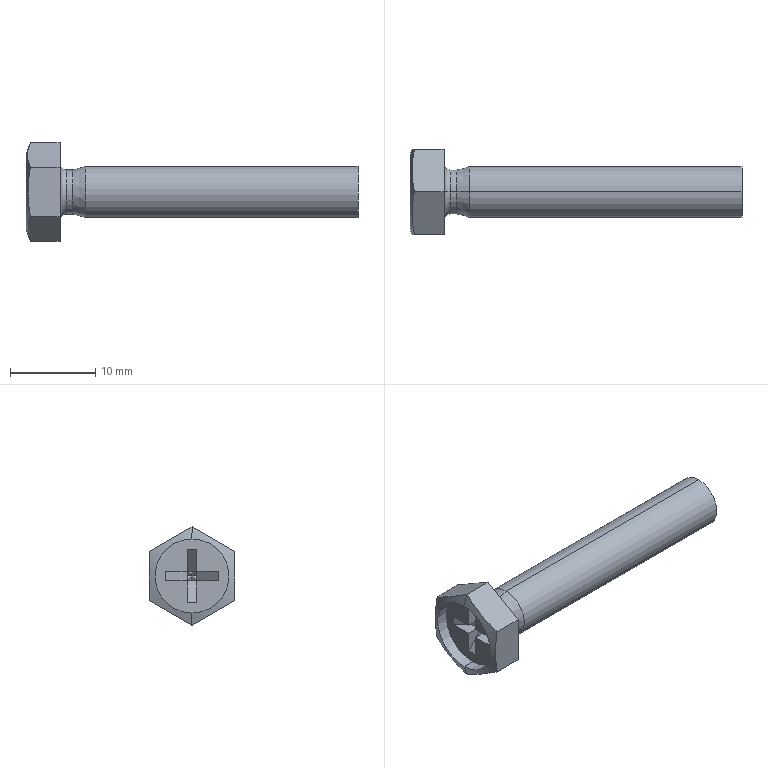Part | SolidWorks | features Cut 2, RevCut 2, CirPattern 1, Extrusion 1, LPattern 1, Revolution 1 | 1 solid | 45 faces | box 39 x 10 x 11.547 mm | volume 1217 mm3 | plane 33 | cylinder 6 | cone 4 | torus 2 | commonest cylinder face diameters 5.2 x2 6 x2 8.7 x2
STEP:
#1=CARTESIAN_POINT('',(1.4,0.,-4.35));
#2=VERTEX_POINT('',#1);
#3=CARTESIAN_POINT('',(1.4,0.,4.35));
#4=VERTEX_POINT('',#3);
#5=CARTESIAN_POINT('',(1.4,0.,0.));
#6=DIRECTION('',(-1.,0.,0.));
#7=DIRECTION('',(0.,0.,1.));
#8=AXIS2_PLACEMENT_3D('',#5,#6,#7);
#9=CIRCLE('',#8,4.35);
#10=EDGE_CURVE('',#2,#4,#9,.T.);
#11=ORIENTED_EDGE('',*,*,#10,.F.);
#12=CARTESIAN_POINT('',(0.,0.,-4.35));
#13=VERTEX_POINT('',#12);
#14=CARTESIAN_POINT('',(1.4,0.,-4.35));
#15=DIRECTION('',(-1.,0.,0.));
#16=VECTOR('',#15,1000.);
#17=LINE('',#14,#16);
#18=EDGE_CURVE('',#2,#13,#17,.T.);
#19=ORIENTED_EDGE('',*,*,#18,.T.);
#20=CARTESIAN_POINT('',(0.,0.,4.35));
#21=VERTEX_POINT('',#20);
#22=CARTESIAN_POINT('',(0.,0.,0.));
#23=DIRECTION('',(-1.,0.,0.));
#24=DIRECTION('',(0.,0.,1.));
#25=AXIS2_PLACEMENT_3D('',#22,#23,#24);
#26=CIRCLE('',#25,4.35);
#27=EDGE_CURVE('',#13,#21,#26,.T.);
#28=ORIENTED_EDGE('',*,*,#27,.T.);
#29=CARTESIAN_POINT('',(1.4,0.,4.35));
#30=DIRECTION('',(-1.,0.,0.));
#31=VECTOR('',#30,1000.);
#32=LINE('',#29,#31);
#33=EDGE_CURVE('',#4,#21,#32,.T.);
#34=ORIENTED_EDGE('',*,*,#33,.F.);
#35=EDGE_LOOP('',(#11,#19,#28,#34));
#36=FACE_OUTER_BOUND('',#35,.T.);
#37=CARTESIAN_POINT('',(1.4,0.,0.));
#38=DIRECTION('',(-1.,0.,0.));
#39=DIRECTION('',(0.,0.,1.));
#40=AXIS2_PLACEMENT_3D('',#37,#38,#39);
#41=CYLINDRICAL_SURFACE('',#40,4.35);
#42=ADVANCED_FACE('',(#36),#41,.F.);
#43=CARTESIAN_POINT('',(0.,0.,0.));
#44=DIRECTION('',(-1.,0.,0.));
#45=DIRECTION('',(0.,0.,1.));
#46=AXIS2_PLACEMENT_3D('',#43,#44,#45);
#47=CIRCLE('',#46,4.35);
#48=EDGE_CURVE('',#21,#13,#47,.T.);
#49=ORIENTED_EDGE('',*,*,#48,.F.);
#50=CARTESIAN_POINT('',(0.5181,0.,5.774));
#51=VERTEX_POINT('',#50);
#52=CARTESIAN_POINT('',(0.,0.,4.35));
#53=DIRECTION('',(0.342,0.,0.9397));
#54=VECTOR('',#53,1000.);
#55=LINE('',#52,#54);
#56=EDGE_CURVE('',#21,#51,#55,.T.);
#57=ORIENTED_EDGE('',*,*,#56,.T.);
#58=CARTESIAN_POINT('',(0.5181,5.,2.887));
#59=VERTEX_POINT('',#58);
#60=CARTESIAN_POINT('',(0.5181,0.,5.774));
#61=CARTESIAN_POINT('',(0.343,0.8333,5.292));
#62=CARTESIAN_POINT('',(0.1302,2.5,4.33));
#63=CARTESIAN_POINT('',(0.343,4.167,3.368));
#64=CARTESIAN_POINT('',(0.5181,5.,2.887));
#65=B_SPLINE_CURVE_WITH_KNOTS('',3,(#60,#61,#62,#63,#64),.UNSPECIFIED.,.F.,.F.,(4,1,4),(0.000000231,0.002887,0.005774),.UNSPECIFIED.);
#66=EDGE_CURVE('',#51,#59,#65,.T.);
#67=ORIENTED_EDGE('',*,*,#66,.T.);
#68=CARTESIAN_POINT('',(0.5181,5.,-2.887));
#69=VERTEX_POINT('',#68);
#70=CARTESIAN_POINT('',(0.5181,5.,2.887));
#71=CARTESIAN_POINT('',(0.3437,5.,1.928));
#72=CARTESIAN_POINT('',(0.2369,5.,0.9672));
#73=CARTESIAN_POINT('',(0.2364,5.,-0.4771));
#74=CARTESIAN_POINT('',(0.2621,5.,-0.9591));
#75=CARTESIAN_POINT('',(0.3594,5.,-1.924));
#76=CARTESIAN_POINT('',(0.431,5.,-2.408));
#77=CARTESIAN_POINT('',(0.5181,5.,-2.887));
#78=B_SPLINE_CURVE_WITH_KNOTS('',3,(#70,#71,#72,#73,#74,#75,#76,#77),.UNSPECIFIED.,.F.,.F.,(4,2,2,4),(0.0105,0.01341,0.01486,0.01631),.UNSPECIFIED.);
#79=EDGE_CURVE('',#59,#69,#78,.T.);
#80=ORIENTED_EDGE('',*,*,#79,.T.);
#81=CARTESIAN_POINT('',(0.5181,0.,-5.774));
#82=VERTEX_POINT('',#81);
#83=CARTESIAN_POINT('',(0.5181,5.,-2.887));
#84=CARTESIAN_POINT('',(0.343,4.167,-3.368));
#85=CARTESIAN_POINT('',(0.1302,2.5,-4.33));
#86=CARTESIAN_POINT('',(0.343,0.8333,-5.292));
#87=CARTESIAN_POINT('',(0.5181,0.,-5.774));
#88=B_SPLINE_CURVE_WITH_KNOTS('',3,(#83,#84,#85,#86,#87),.UNSPECIFIED.,.F.,.F.,(4,1,4),(0.000000231,0.002887,0.005774),.UNSPECIFIED.);
#89=EDGE_CURVE('',#69,#82,#88,.T.);
#90=ORIENTED_EDGE('',*,*,#89,.T.);
#91=CARTESIAN_POINT('',(0.,0.,-4.35));
#92=DIRECTION('',(0.342,0.,-0.9397));
#93=VECTOR('',#92,1000.);
#94=LINE('',#91,#93);
#95=EDGE_CURVE('',#13,#82,#94,.T.);
#96=ORIENTED_EDGE('',*,*,#95,.F.);
#97=EDGE_LOOP('',(#49,#57,#67,#80,#90,#96));
#98=FACE_OUTER_BOUND('',#97,.T.);
#99=CARTESIAN_POINT('',(0.,0.,0.));
#100=DIRECTION('',(1.,0.,0.));
#101=DIRECTION('',(0.,0.,-1.));
#102=AXIS2_PLACEMENT_3D('',#99,#100,#101);
#103=CONICAL_SURFACE('',#102,4.35,1.222);
#104=ADVANCED_FACE('',(#98),#103,.T.);
#105=CARTESIAN_POINT('',(4.,0.,-3.4));
#106=VERTEX_POINT('',#105);
#107=CARTESIAN_POINT('',(4.,0.,3.4));
#108=VERTEX_POINT('',#107);
#109=CARTESIAN_POINT('',(4.,0.,0.));
#110=DIRECTION('',(-1.,0.,0.));
#111=DIRECTION('',(0.,0.,1.));
#112=AXIS2_PLACEMENT_3D('',#109,#110,#111);
#113=CIRCLE('',#112,3.4);
#114=EDGE_CURVE('',#106,#108,#113,.T.);
#115=ORIENTED_EDGE('',*,*,#114,.F.);
#116=CARTESIAN_POINT('',(4.8,0.,-2.6));
#117=VERTEX_POINT('',#116);
#118=CARTESIAN_POINT('',(4.8,0.,-3.4));
#119=DIRECTION('',(0.,1.,0.));
#120=DIRECTION('',(0.,0.,1.));
#121=AXIS2_PLACEMENT_3D('',#118,#119,#120);
#122=CIRCLE('',#121,0.8);
#123=EDGE_CURVE('',#106,#117,#122,.T.);
#124=ORIENTED_EDGE('',*,*,#123,.T.);
#125=CARTESIAN_POINT('',(4.8,0.,2.6));
#126=VERTEX_POINT('',#125);
#127=CARTESIAN_POINT('',(4.8,0.,0.));
#128=DIRECTION('',(-1.,0.,0.));
#129=DIRECTION('',(0.,0.,1.));
#130=AXIS2_PLACEMENT_3D('',#127,#128,#129);
#131=CIRCLE('',#130,2.6);
#132=EDGE_CURVE('',#117,#126,#131,.T.);
#133=ORIENTED_EDGE('',*,*,#132,.T.);
#134=CARTESIAN_POINT('',(4.8,0.,3.4));
#135=DIRECTION('',(0.,-1.,0.));
#136=DIRECTION('',(0.,0.,-1.));
#137=AXIS2_PLACEMENT_3D('',#134,#135,#136);
#138=CIRCLE('',#137,0.8);
#139=EDGE_CURVE('',#108,#126,#138,.T.);
#140=ORIENTED_EDGE('',*,*,#139,.F.);
#141=EDGE_LOOP('',(#115,#124,#133,#140));
#142=FACE_OUTER_BOUND('',#141,.T.);
#143=CARTESIAN_POINT('',(4.8,0.,0.));
#144=DIRECTION('',(-1.,0.,0.));
#145=DIRECTION('',(0.,0.,1.));
#146=AXIS2_PLACEMENT_3D('',#143,#144,#145);
#147=TOROIDAL_SURFACE('',#146,3.4,0.8);
#148=ADVANCED_FACE('',(#142),#147,.F.);
#149=CARTESIAN_POINT('',(5.507,0.,2.6));
#150=VERTEX_POINT('',#149);
#151=CARTESIAN_POINT('',(5.507,0.,-2.6));
#152=VERTEX_POINT('',#151);
#153=CARTESIAN_POINT('',(5.507,0.,0.));
#154=DIRECTION('',(-1.,0.,0.));
#155=DIRECTION('',(0.,0.,1.));
#156=AXIS2_PLACEMENT_3D('',#153,#154,#155);
#157=CIRCLE('',#156,2.6);
#158=EDGE_CURVE('',#150,#152,#157,.T.);
#159=ORIENTED_EDGE('',*,*,#158,.T.);
#160=CARTESIAN_POINT('',(0.,0.,-2.6));
#161=DIRECTION('',(-1.,0.,0.));
#162=VECTOR('',#161,1000.);
#163=LINE('',#160,#162);
#164=EDGE_CURVE('',#152,#117,#163,.T.);
#165=ORIENTED_EDGE('',*,*,#164,.T.);
#166=CARTESIAN_POINT('',(4.8,0.,0.));
#167=DIRECTION('',(-1.,0.,0.));
#168=DIRECTION('',(0.,0.,1.));
#169=AXIS2_PLACEMENT_3D('',#166,#167,#168);
#170=CIRCLE('',#169,2.6);
#171=EDGE_CURVE('',#126,#117,#170,.T.);
#172=ORIENTED_EDGE('',*,*,#171,.F.);
#173=CARTESIAN_POINT('',(0.,0.,2.6));
#174=DIRECTION('',(-1.,0.,0.));
#175=VECTOR('',#174,1000.);
#176=LINE('',#173,#175);
#177=EDGE_CURVE('',#150,#126,#176,.T.);
#178=ORIENTED_EDGE('',*,*,#177,.F.);
#179=EDGE_LOOP('',(#159,#165,#172,#178));
#180=FACE_OUTER_BOUND('',#179,.T.);
#181=CARTESIAN_POINT('',(0.,0.,0.));
#182=DIRECTION('',(-1.,0.,0.));
#183=DIRECTION('',(0.,0.,1.));
#184=AXIS2_PLACEMENT_3D('',#181,#182,#183);
#185=CYLINDRICAL_SURFACE('',#184,2.6);
#186=ADVANCED_FACE('',(#180),#185,.T.);
#187=ORIENTED_EDGE('',*,*,#158,.F.);
#188=CARTESIAN_POINT('',(7.,0.,3.));
#189=VERTEX_POINT('',#188);
#190=CARTESIAN_POINT('',(7.,0.,3.));
#191=DIRECTION('',(0.9659,0.,0.2588));
#192=VECTOR('',#191,1000.);
#193=LINE('',#190,#192);
#194=EDGE_CURVE('',#150,#189,#193,.T.);
#195=ORIENTED_EDGE('',*,*,#194,.T.);
#196=CARTESIAN_POINT('',(7.,0.,-3.));
#197=VERTEX_POINT('',#196);
#198=CARTESIAN_POINT('',(7.,0.,0.));
#199=DIRECTION('',(-1.,0.,0.));
#200=DIRECTION('',(0.,0.,1.));
#201=AXIS2_PLACEMENT_3D('',#198,#199,#200);
#202=CIRCLE('',#201,3.);
#203=EDGE_CURVE('',#189,#197,#202,.T.);
#204=ORIENTED_EDGE('',*,*,#203,.T.);
#205=CARTESIAN_POINT('',(7.,0.,-3.));
#206=DIRECTION('',(0.9659,0.,-0.2588));
#207=VECTOR('',#206,1000.);
#208=LINE('',#205,#207);
#209=EDGE_CURVE('',#152,#197,#208,.T.);
#210=ORIENTED_EDGE('',*,*,#209,.F.);
#211=EDGE_LOOP('',(#187,#195,#204,#210));
#212=FACE_OUTER_BOUND('',#211,.T.);
#213=CARTESIAN_POINT('',(7.,0.,0.));
#214=DIRECTION('',(1.,0.,0.));
#215=DIRECTION('',(0.,0.,-1.));
#216=AXIS2_PLACEMENT_3D('',#213,#214,#215);
#217=CONICAL_SURFACE('',#216,3.,0.2618);
#218=ADVANCED_FACE('',(#212),#217,.T.);
#219=CARTESIAN_POINT('',(39.,0.,3.));
#220=VERTEX_POINT('',#219);
#221=CARTESIAN_POINT('',(39.,0.,-3.));
#222=VERTEX_POINT('',#221);
#223=CARTESIAN_POINT('',(39.,0.,0.));
#224=DIRECTION('',(-1.,0.,0.));
#225=DIRECTION('',(0.,0.,1.));
#226=AXIS2_PLACEMENT_3D('',#223,#224,#225);
#227=CIRCLE('',#226,3.);
#228=EDGE_CURVE('',#220,#222,#227,.T.);
#229=ORIENTED_EDGE('',*,*,#228,.T.);
#230=CARTESIAN_POINT('',(0.,0.,-3.));
#231=DIRECTION('',(-1.,0.,0.));
#232=VECTOR('',#231,1000.);
#233=LINE('',#230,#232);
#234=EDGE_CURVE('',#222,#197,#233,.T.);
#235=ORIENTED_EDGE('',*,*,#234,.T.);
#236=ORIENTED_EDGE('',*,*,#203,.F.);
#237=CARTESIAN_POINT('',(0.,0.,3.));
#238=DIRECTION('',(-1.,0.,0.));
#239=VECTOR('',#238,1000.);
#240=LINE('',#237,#239);
#241=EDGE_CURVE('',#220,#189,#240,.T.);
#242=ORIENTED_EDGE('',*,*,#241,.F.);
#243=EDGE_LOOP('',(#229,#235,#236,#242));
#244=FACE_OUTER_BOUND('',#243,.T.);
#245=CARTESIAN_POINT('',(0.,0.,0.));
#246=DIRECTION('',(-1.,0.,0.));
#247=DIRECTION('',(0.,0.,1.));
#248=AXIS2_PLACEMENT_3D('',#245,#246,#247);
#249=CYLINDRICAL_SURFACE('',#248,3.);
#250=ADVANCED_FACE('',(#244),#249,.T.);
#251=CARTESIAN_POINT('',(1.4,0.,0.));
#252=DIRECTION('',(-1.,0.,0.));
#253=DIRECTION('',(0.,0.,1.));
#254=AXIS2_PLACEMENT_3D('',#251,#252,#253);
#255=CIRCLE('',#254,4.35);
#256=EDGE_CURVE('',#4,#2,#255,.T.);
#257=ORIENTED_EDGE('',*,*,#256,.T.);
#258=ORIENTED_EDGE('',*,*,#10,.T.);
#259=EDGE_LOOP('',(#257,#258));
#260=FACE_OUTER_BOUND('',#259,.T.);
#261=CARTESIAN_POINT('',(1.4,3.1,0.572));
#262=VERTEX_POINT('',#261);
#263=CARTESIAN_POINT('',(1.4,3.1,-0.572));
#264=VERTEX_POINT('',#263);
#265=CARTESIAN_POINT('',(1.4,3.1,0.));
#266=DIRECTION('',(0.,0.,-1.));
#267=VECTOR('',#266,1000.);
#268=LINE('',#265,#267);
#269=EDGE_CURVE('',#262,#264,#268,.T.);
#270=ORIENTED_EDGE('',*,*,#269,.F.);
#271=CARTESIAN_POINT('',(1.4,0.572,0.572));
#272=VERTEX_POINT('',#271);
#273=CARTESIAN_POINT('',(1.4,0.,0.572));
#274=DIRECTION('',(0.,-1.,0.));
#275=VECTOR('',#274,1000.);
#276=LINE('',#273,#275);
#277=EDGE_CURVE('',#262,#272,#276,.T.);
#278=ORIENTED_EDGE('',*,*,#277,.T.);
#279=CARTESIAN_POINT('',(1.4,0.572,3.1));
#280=VERTEX_POINT('',#279);
#281=CARTESIAN_POINT('',(1.4,0.572,0.));
#282=DIRECTION('',(0.,0.,-1.));
#283=VECTOR('',#282,1000.);
#284=LINE('',#281,#283);
#285=EDGE_CURVE('',#280,#272,#284,.T.);
#286=ORIENTED_EDGE('',*,*,#285,.F.);
#287=CARTESIAN_POINT('',(1.4,-0.572,3.1));
#288=VERTEX_POINT('',#287);
#289=CARTESIAN_POINT('',(1.4,0.,3.1));
#290=DIRECTION('',(0.,1.,0.));
#291=VECTOR('',#290,1000.);
#292=LINE('',#289,#291);
#293=EDGE_CURVE('',#288,#280,#292,.T.);
#294=ORIENTED_EDGE('',*,*,#293,.F.);
#295=CARTESIAN_POINT('',(1.4,-0.572,0.572));
#296=VERTEX_POINT('',#295);
#297=CARTESIAN_POINT('',(1.4,-0.572,0.));
#298=DIRECTION('',(0.,0.,-1.));
#299=VECTOR('',#298,1000.);
#300=LINE('',#297,#299);
#301=EDGE_CURVE('',#288,#296,#300,.T.);
#302=ORIENTED_EDGE('',*,*,#301,.T.);
#303=CARTESIAN_POINT('',(1.4,-3.1,0.572));
#304=VERTEX_POINT('',#303);
#305=CARTESIAN_POINT('',(1.4,0.,0.572));
#306=DIRECTION('',(0.,-1.,0.));
#307=VECTOR('',#306,1000.);
#308=LINE('',#305,#307);
#309=EDGE_CURVE('',#296,#304,#308,.T.);
#310=ORIENTED_EDGE('',*,*,#309,.T.);
#311=CARTESIAN_POINT('',(1.4,-3.1,-0.572));
#312=VERTEX_POINT('',#311);
#313=CARTESIAN_POINT('',(1.4,-3.1,0.));
#314=DIRECTION('',(0.,0.,1.));
#315=VECTOR('',#314,1000.);
#316=LINE('',#313,#315);
#317=EDGE_CURVE('',#312,#304,#316,.T.);
#318=ORIENTED_EDGE('',*,*,#317,.F.);
#319=CARTESIAN_POINT('',(1.4,-0.572,-0.572));
#320=VERTEX_POINT('',#319);
#321=CARTESIAN_POINT('',(1.4,0.,-0.572));
#322=DIRECTION('',(0.,-1.,0.));
#323=VECTOR('',#322,1000.);
#324=LINE('',#321,#323);
#325=EDGE_CURVE('',#320,#312,#324,.T.);
#326=ORIENTED_EDGE('',*,*,#325,.F.);
#327=CARTESIAN_POINT('',(1.4,-0.572,-3.1));
#328=VERTEX_POINT('',#327);
#329=CARTESIAN_POINT('',(1.4,-0.572,0.));
#330=DIRECTION('',(0.,0.,-1.));
#331=VECTOR('',#330,1000.);
#332=LINE('',#329,#331);
#333=EDGE_CURVE('',#320,#328,#332,.T.);
#334=ORIENTED_EDGE('',*,*,#333,.T.);
#335=CARTESIAN_POINT('',(1.4,0.572,-3.1));
#336=VERTEX_POINT('',#335);
#337=CARTESIAN_POINT('',(1.4,0.,-3.1));
#338=DIRECTION('',(0.,-1.,0.));
#339=VECTOR('',#338,1000.);
#340=LINE('',#337,#339);
#341=EDGE_CURVE('',#336,#328,#340,.T.);
#342=ORIENTED_EDGE('',*,*,#341,.F.);
#343=CARTESIAN_POINT('',(1.4,0.572,-0.572));
#344=VERTEX_POINT('',#343);
#345=CARTESIAN_POINT('',(1.4,0.572,0.));
#346=DIRECTION('',(0.,0.,-1.));
#347=VECTOR('',#346,1000.);
#348=LINE('',#345,#347);
#349=EDGE_CURVE('',#344,#336,#348,.T.);
#350=ORIENTED_EDGE('',*,*,#349,.F.);
#351=CARTESIAN_POINT('',(1.4,0.,-0.572));
#352=DIRECTION('',(0.,-1.,0.));
#353=VECTOR('',#352,1000.);
#354=LINE('',#351,#353);
#355=EDGE_CURVE('',#264,#344,#354,.T.);
#356=ORIENTED_EDGE('',*,*,#355,.F.);
#357=EDGE_LOOP('',(#270,#278,#286,#294,#302,#310,#318,#326,#334,#342,#350,#356));
#358=FACE_BOUND('',#357,.T.);
#359=CARTESIAN_POINT('',(1.4,0.,0.));
#360=DIRECTION('',(-1.,0.,0.));
#361=DIRECTION('',(0.,0.,1.));
#362=AXIS2_PLACEMENT_3D('',#359,#360,#361);
#363=PLANE('',#362);
#364=ADVANCED_FACE('',(#260,#358),#363,.T.);
#365=CARTESIAN_POINT('',(3.732,-0.572,0.572));
#366=VERTEX_POINT('',#365);
#367=CARTESIAN_POINT('',(3.732,0.572,0.572));
#368=VERTEX_POINT('',#367);
#369=CARTESIAN_POINT('',(3.732,-0.572,0.572));
#370=DIRECTION('',(0.,1.,0.));
#371=VECTOR('',#370,1000.);
#372=LINE('',#369,#371);
#373=EDGE_CURVE('',#366,#368,#372,.T.);
#374=ORIENTED_EDGE('',*,*,#373,.F.);
#375=CARTESIAN_POINT('',(0.9,-0.572,3.642));
#376=DIRECTION('',(0.6781,0.,-0.735));
#377=VECTOR('',#376,1000.);
#378=LINE('',#375,#377);
#379=EDGE_CURVE('',#288,#366,#378,.T.);
#380=ORIENTED_EDGE('',*,*,#379,.F.);
#381=ORIENTED_EDGE('',*,*,#293,.T.);
#382=CARTESIAN_POINT('',(0.9,0.572,3.642));
#383=DIRECTION('',(0.6781,0.,-0.735));
#384=VECTOR('',#383,1000.);
#385=LINE('',#382,#384);
#386=EDGE_CURVE('',#280,#368,#385,.T.);
#387=ORIENTED_EDGE('',*,*,#386,.T.);
#388=EDGE_LOOP('',(#374,#380,#381,#387));
#389=FACE_OUTER_BOUND('',#388,.T.);
#390=CARTESIAN_POINT('',(0.9,-0.572,3.642));
#391=DIRECTION('',(0.735,0.,0.6781));
#392=DIRECTION('',(0.6781,0.,-0.735));
#393=AXIS2_PLACEMENT_3D('',#390,#391,#392);
#394=PLANE('',#393);
#395=ADVANCED_FACE('',(#389),#394,.F.);
#396=ORIENTED_EDGE('',*,*,#379,.T.);
#397=CARTESIAN_POINT('',(4.26,-0.572,0.572));
#398=DIRECTION('',(-1.,0.,0.));
#399=VECTOR('',#398,1000.);
#400=LINE('',#397,#399);
#401=EDGE_CURVE('',#366,#296,#400,.T.);
#402=ORIENTED_EDGE('',*,*,#401,.T.);
#403=ORIENTED_EDGE('',*,*,#301,.F.);
#404=EDGE_LOOP('',(#396,#402,#403));
#405=FACE_OUTER_BOUND('',#404,.T.);
#406=CARTESIAN_POINT('',(4.26,-0.572,0.));
#407=DIRECTION('',(0.,1.,0.));
#408=DIRECTION('',(0.,0.,1.));
#409=AXIS2_PLACEMENT_3D('',#406,#407,#408);
#410=PLANE('',#409);
#411=ADVANCED_FACE('',(#405),#410,.T.);
#412=CARTESIAN_POINT('',(4.26,0.572,0.572));
#413=DIRECTION('',(-1.,0.,0.));
#414=VECTOR('',#413,1000.);
#415=LINE('',#412,#414);
#416=EDGE_CURVE('',#368,#272,#415,.T.);
#417=ORIENTED_EDGE('',*,*,#416,.F.);
#418=ORIENTED_EDGE('',*,*,#386,.F.);
#419=ORIENTED_EDGE('',*,*,#285,.T.);
#420=EDGE_LOOP('',(#417,#418,#419));
#421=FACE_OUTER_BOUND('',#420,.T.);
#422=CARTESIAN_POINT('',(4.26,0.572,0.));
#423=DIRECTION('',(0.,1.,0.));
#424=DIRECTION('',(0.,0.,1.));
#425=AXIS2_PLACEMENT_3D('',#422,#423,#424);
#426=PLANE('',#425);
#427=ADVANCED_FACE('',(#421),#426,.F.);
#428=CARTESIAN_POINT('',(0.5181,-5.,-2.887));
#429=VERTEX_POINT('',#428);
#430=CARTESIAN_POINT('',(0.5181,-5.,2.887));
#431=VERTEX_POINT('',#430);
#432=CARTESIAN_POINT('',(0.5181,-5.,-2.887));
#433=CARTESIAN_POINT('',(0.431,-5.,-2.408));
#434=CARTESIAN_POINT('',(0.3594,-5.,-1.924));
#435=CARTESIAN_POINT('',(0.2621,-5.,-0.9591));
#436=CARTESIAN_POINT('',(0.2364,-5.,-0.4771));
#437=CARTESIAN_POINT('',(0.2369,-5.,0.9672));
#438=CARTESIAN_POINT('',(0.3437,-5.,1.928));
#439=CARTESIAN_POINT('',(0.5181,-5.,2.887));
#440=B_SPLINE_CURVE_WITH_KNOTS('',3,(#432,#433,#434,#435,#436,#437,#438,#439),.UNSPECIFIED.,.F.,.F.,(4,2,2,4),(0.004887,0.006344,0.007801,0.01071),.UNSPECIFIED.);
#441=EDGE_CURVE('',#429,#431,#440,.T.);
#442=ORIENTED_EDGE('',*,*,#441,.F.);
#443=CARTESIAN_POINT('',(4.,-5.,-2.887));
#444=VERTEX_POINT('',#443);
#445=CARTESIAN_POINT('',(4.,-5.,-2.887));
#446=DIRECTION('',(-1.,0.,0.));
#447=VECTOR('',#446,1000.);
#448=LINE('',#445,#447);
#449=EDGE_CURVE('',#444,#429,#448,.T.);
#450=ORIENTED_EDGE('',*,*,#449,.F.);
#451=CARTESIAN_POINT('',(4.,-5.,2.887));
#452=VERTEX_POINT('',#451);
#453=CARTESIAN_POINT('',(4.,-5.,2.887));
#454=DIRECTION('',(0.,0.,-1.));
#455=VECTOR('',#454,1000.);
#456=LINE('',#453,#455);
#457=EDGE_CURVE('',#452,#444,#456,.T.);
#458=ORIENTED_EDGE('',*,*,#457,.F.);
#459=CARTESIAN_POINT('',(4.,-5.,2.887));
#460=DIRECTION('',(-1.,0.,0.));
#461=VECTOR('',#460,1000.);
#462=LINE('',#459,#461);
#463=EDGE_CURVE('',#452,#431,#462,.T.);
#464=ORIENTED_EDGE('',*,*,#463,.T.);
#465=EDGE_LOOP('',(#442,#450,#458,#464));
#466=FACE_OUTER_BOUND('',#465,.T.);
#467=CARTESIAN_POINT('',(4.,-5.,2.887));
#468=DIRECTION('',(0.,1.,0.));
#469=DIRECTION('',(0.,0.,1.));
#470=AXIS2_PLACEMENT_3D('',#467,#468,#469);
#471=PLANE('',#470);
#472=ADVANCED_FACE('',(#466),#471,.F.);
#473=CARTESIAN_POINT('',(0.5181,0.,-5.774));
#474=CARTESIAN_POINT('',(0.343,-0.8333,-5.292));
#475=CARTESIAN_POINT('',(0.1302,-2.5,-4.33));
#476=CARTESIAN_POINT('',(0.343,-4.167,-3.368));
#477=CARTESIAN_POINT('',(0.5181,-5.,-2.887));
#478=B_SPLINE_CURVE_WITH_KNOTS('',3,(#473,#474,#475,#476,#477),.UNSPECIFIED.,.F.,.F.,(4,1,4),(0.000000231,0.002887,0.005774),.UNSPECIFIED.);
#479=EDGE_CURVE('',#82,#429,#478,.T.);
#480=ORIENTED_EDGE('',*,*,#479,.F.);
#481=CARTESIAN_POINT('',(4.,0.,-5.774));
#482=VERTEX_POINT('',#481);
#483=CARTESIAN_POINT('',(4.,0.,-5.774));
#484=DIRECTION('',(-1.,0.,0.));
#485=VECTOR('',#484,1000.);
#486=LINE('',#483,#485);
#487=EDGE_CURVE('',#482,#82,#486,.T.);
#488=ORIENTED_EDGE('',*,*,#487,.F.);
#489=CARTESIAN_POINT('',(4.,-5.,-2.887));
#490=DIRECTION('',(0.,0.866,-0.5));
#491=VECTOR('',#490,1000.);
#492=LINE('',#489,#491);
#493=EDGE_CURVE('',#444,#482,#492,.T.);
#494=ORIENTED_EDGE('',*,*,#493,.F.);
#495=ORIENTED_EDGE('',*,*,#449,.T.);
#496=EDGE_LOOP('',(#480,#488,#494,#495));
#497=FACE_OUTER_BOUND('',#496,.T.);
#498=CARTESIAN_POINT('',(4.,-5.,-2.887));
#499=DIRECTION('',(0.,0.5,0.866));
#500=DIRECTION('',(0.,-0.866,0.5));
#501=AXIS2_PLACEMENT_3D('',#498,#499,#500);
#502=PLANE('',#501);
#503=ADVANCED_FACE('',(#497),#502,.F.);
#504=ORIENTED_EDGE('',*,*,#89,.F.);
#505=CARTESIAN_POINT('',(4.,5.,-2.887));
#506=VERTEX_POINT('',#505);
#507=CARTESIAN_POINT('',(4.,5.,-2.887));
#508=DIRECTION('',(-1.,0.,0.));
#509=VECTOR('',#508,1000.);
#510=LINE('',#507,#509);
#511=EDGE_CURVE('',#506,#69,#510,.T.);
#512=ORIENTED_EDGE('',*,*,#511,.F.);
#513=CARTESIAN_POINT('',(4.,0.,-5.774));
#514=DIRECTION('',(0.,0.866,0.5));
#515=VECTOR('',#514,1000.);
#516=LINE('',#513,#515);
#517=EDGE_CURVE('',#482,#506,#516,.T.);
#518=ORIENTED_EDGE('',*,*,#517,.F.);
#519=ORIENTED_EDGE('',*,*,#487,.T.);
#520=EDGE_LOOP('',(#504,#512,#518,#519));
#521=FACE_OUTER_BOUND('',#520,.T.);
#522=CARTESIAN_POINT('',(4.,0.,-5.774));
#523=DIRECTION('',(0.,-0.5,0.866));
#524=DIRECTION('',(0.,-0.866,-0.5));
#525=AXIS2_PLACEMENT_3D('',#522,#523,#524);
#526=PLANE('',#525);
#527=ADVANCED_FACE('',(#521),#526,.F.);
#528=ORIENTED_EDGE('',*,*,#79,.F.);
#529=CARTESIAN_POINT('',(4.,5.,2.887));
#530=VERTEX_POINT('',#529);
#531=CARTESIAN_POINT('',(4.,5.,2.887));
#532=DIRECTION('',(-1.,0.,0.));
#533=VECTOR('',#532,1000.);
#534=LINE('',#531,#533);
#535=EDGE_CURVE('',#530,#59,#534,.T.);
#536=ORIENTED_EDGE('',*,*,#535,.F.);
#537=CARTESIAN_POINT('',(4.,5.,-2.887));
#538=DIRECTION('',(0.,0.,1.));
#539=VECTOR('',#538,1000.);
#540=LINE('',#537,#539);
#541=EDGE_CURVE('',#506,#530,#540,.T.);
#542=ORIENTED_EDGE('',*,*,#541,.F.);
#543=ORIENTED_EDGE('',*,*,#511,.T.);
#544=EDGE_LOOP('',(#528,#536,#542,#543));
#545=FACE_OUTER_BOUND('',#544,.T.);
#546=CARTESIAN_POINT('',(4.,5.,-2.887));
#547=DIRECTION('',(0.,-1.,0.));
#548=DIRECTION('',(0.,0.,-1.));
#549=AXIS2_PLACEMENT_3D('',#546,#547,#548);
#550=PLANE('',#549);
#551=ADVANCED_FACE('',(#545),#550,.F.);
#552=ORIENTED_EDGE('',*,*,#66,.F.);
#553=CARTESIAN_POINT('',(4.,0.,5.774));
#554=VERTEX_POINT('',#553);
#555=CARTESIAN_POINT('',(4.,0.,5.774));
#556=DIRECTION('',(-1.,0.,0.));
#557=VECTOR('',#556,1000.);
#558=LINE('',#555,#557);
#559=EDGE_CURVE('',#554,#51,#558,.T.);
#560=ORIENTED_EDGE('',*,*,#559,.F.);
#561=CARTESIAN_POINT('',(4.,5.,2.887));
#562=DIRECTION('',(0.,-0.866,0.5));
#563=VECTOR('',#562,1000.);
#564=LINE('',#561,#563);
#565=EDGE_CURVE('',#530,#554,#564,.T.);
#566=ORIENTED_EDGE('',*,*,#565,.F.);
#567=ORIENTED_EDGE('',*,*,#535,.T.);
#568=EDGE_LOOP('',(#552,#560,#566,#567));
#569=FACE_OUTER_BOUND('',#568,.T.);
#570=CARTESIAN_POINT('',(4.,5.,2.887));
#571=DIRECTION('',(0.,-0.5,-0.866));
#572=DIRECTION('',(0.,0.866,-0.5));
#573=AXIS2_PLACEMENT_3D('',#570,#571,#572);
#574=PLANE('',#573);
#575=ADVANCED_FACE('',(#569),#574,.F.);
#576=CARTESIAN_POINT('',(0.5181,-5.,2.887));
#577=CARTESIAN_POINT('',(0.343,-4.167,3.368));
#578=CARTESIAN_POINT('',(0.1302,-2.5,4.33));
#579=CARTESIAN_POINT('',(0.343,-0.8333,5.292));
#580=CARTESIAN_POINT('',(0.5181,0.,5.774));
#581=B_SPLINE_CURVE_WITH_KNOTS('',3,(#576,#577,#578,#579,#580),.UNSPECIFIED.,.F.,.F.,(4,1,4),(0.000000231,0.002887,0.005774),.UNSPECIFIED.);
#582=EDGE_CURVE('',#431,#51,#581,.T.);
#583=ORIENTED_EDGE('',*,*,#582,.F.);
#584=ORIENTED_EDGE('',*,*,#463,.F.);
#585=CARTESIAN_POINT('',(4.,0.,5.774));
#586=DIRECTION('',(0.,-0.866,-0.5));
#587=VECTOR('',#586,1000.);
#588=LINE('',#585,#587);
#589=EDGE_CURVE('',#554,#452,#588,.T.);
#590=ORIENTED_EDGE('',*,*,#589,.F.);
#591=ORIENTED_EDGE('',*,*,#559,.T.);
#592=EDGE_LOOP('',(#583,#584,#590,#591));
#593=FACE_OUTER_BOUND('',#592,.T.);
#594=CARTESIAN_POINT('',(4.,0.,5.774));
#595=DIRECTION('',(0.,0.5,-0.866));
#596=DIRECTION('',(0.,0.866,0.5));
#597=AXIS2_PLACEMENT_3D('',#594,#595,#596);
#598=PLANE('',#597);
#599=ADVANCED_FACE('',(#593),#598,.F.);
#600=ORIENTED_EDGE('',*,*,#457,.T.);
#601=ORIENTED_EDGE('',*,*,#493,.T.);
#602=ORIENTED_EDGE('',*,*,#517,.T.);
#603=ORIENTED_EDGE('',*,*,#541,.T.);
#604=ORIENTED_EDGE('',*,*,#565,.T.);
#605=ORIENTED_EDGE('',*,*,#589,.T.);
#606=EDGE_LOOP('',(#600,#601,#602,#603,#604,#605));
#607=FACE_OUTER_BOUND('',#606,.T.);
#608=CARTESIAN_POINT('',(4.,0.,0.));
#609=DIRECTION('',(-1.,0.,0.));
#610=DIRECTION('',(0.,0.,1.));
#611=AXIS2_PLACEMENT_3D('',#608,#609,#610);
#612=CIRCLE('',#611,3.4);
#613=EDGE_CURVE('',#108,#106,#612,.T.);
#614=ORIENTED_EDGE('',*,*,#613,.T.);
#615=ORIENTED_EDGE('',*,*,#114,.T.);
#616=EDGE_LOOP('',(#614,#615));
#617=FACE_BOUND('',#616,.T.);
#618=CARTESIAN_POINT('',(4.,-5.,-2.887));
#619=DIRECTION('',(1.,0.,0.));
#620=DIRECTION('',(0.,0.,-1.));
#621=AXIS2_PLACEMENT_3D('',#618,#619,#620);
#622=PLANE('',#621);
#623=ADVANCED_FACE('',(#607,#617),#622,.T.);
#624=ORIENTED_EDGE('',*,*,#228,.F.);
#625=CARTESIAN_POINT('',(39.,0.,0.));
#626=DIRECTION('',(-1.,0.,0.));
#627=DIRECTION('',(0.,0.,1.));
#628=AXIS2_PLACEMENT_3D('',#625,#626,#627);
#629=CIRCLE('',#628,3.);
#630=EDGE_CURVE('',#222,#220,#629,.T.);
#631=ORIENTED_EDGE('',*,*,#630,.F.);
#632=EDGE_LOOP('',(#624,#631));
#633=FACE_OUTER_BOUND('',#632,.T.);
#634=CARTESIAN_POINT('',(39.,0.,0.));
#635=DIRECTION('',(-1.,0.,0.));
#636=DIRECTION('',(0.,0.,1.));
#637=AXIS2_PLACEMENT_3D('',#634,#635,#636);
#638=PLANE('',#637);
#639=ADVANCED_FACE('',(#633),#638,.F.);
#640=ORIENTED_EDGE('',*,*,#234,.F.);
#641=ORIENTED_EDGE('',*,*,#630,.T.);
#642=ORIENTED_EDGE('',*,*,#241,.T.);
#643=CARTESIAN_POINT('',(7.,0.,0.));
#644=DIRECTION('',(-1.,0.,0.));
#645=DIRECTION('',(0.,0.,1.));
#646=AXIS2_PLACEMENT_3D('',#643,#644,#645);
#647=CIRCLE('',#646,3.);
#648=EDGE_CURVE('',#197,#189,#647,.T.);
#649=ORIENTED_EDGE('',*,*,#648,.F.);
#650=EDGE_LOOP('',(#640,#641,#642,#649));
#651=FACE_OUTER_BOUND('',#650,.T.);
#652=CARTESIAN_POINT('',(0.,0.,0.));
#653=DIRECTION('',(-1.,0.,0.));
#654=DIRECTION('',(0.,0.,1.));
#655=AXIS2_PLACEMENT_3D('',#652,#653,#654);
#656=CYLINDRICAL_SURFACE('',#655,3.);
#657=ADVANCED_FACE('',(#651),#656,.T.);
#658=ORIENTED_EDGE('',*,*,#194,.F.);
#659=CARTESIAN_POINT('',(5.507,0.,0.));
#660=DIRECTION('',(-1.,0.,0.));
#661=DIRECTION('',(0.,0.,1.));
#662=AXIS2_PLACEMENT_3D('',#659,#660,#661);
#663=CIRCLE('',#662,2.6);
#664=EDGE_CURVE('',#152,#150,#663,.T.);
#665=ORIENTED_EDGE('',*,*,#664,.F.);
#666=ORIENTED_EDGE('',*,*,#209,.T.);
#667=ORIENTED_EDGE('',*,*,#648,.T.);
#668=EDGE_LOOP('',(#658,#665,#666,#667));
#669=FACE_OUTER_BOUND('',#668,.T.);
#670=CARTESIAN_POINT('',(7.,0.,0.));
#671=DIRECTION('',(1.,0.,0.));
#672=DIRECTION('',(0.,0.,-1.));
#673=AXIS2_PLACEMENT_3D('',#670,#671,#672);
#674=CONICAL_SURFACE('',#673,3.,0.2618);
#675=ADVANCED_FACE('',(#669),#674,.T.);
#676=ORIENTED_EDGE('',*,*,#164,.F.);
#677=ORIENTED_EDGE('',*,*,#664,.T.);
#678=ORIENTED_EDGE('',*,*,#177,.T.);
#679=ORIENTED_EDGE('',*,*,#132,.F.);
#680=EDGE_LOOP('',(#676,#677,#678,#679));
#681=FACE_OUTER_BOUND('',#680,.T.);
#682=CARTESIAN_POINT('',(0.,0.,0.));
#683=DIRECTION('',(-1.,0.,0.));
#684=DIRECTION('',(0.,0.,1.));
#685=AXIS2_PLACEMENT_3D('',#682,#683,#684);
#686=CYLINDRICAL_SURFACE('',#685,2.6);
#687=ADVANCED_FACE('',(#681),#686,.T.);
#688=ORIENTED_EDGE('',*,*,#123,.F.);
#689=ORIENTED_EDGE('',*,*,#613,.F.);
#690=ORIENTED_EDGE('',*,*,#139,.T.);
#691=ORIENTED_EDGE('',*,*,#171,.T.);
#692=EDGE_LOOP('',(#688,#689,#690,#691));
#693=FACE_OUTER_BOUND('',#692,.T.);
#694=CARTESIAN_POINT('',(4.8,0.,0.));
#695=DIRECTION('',(-1.,0.,0.));
#696=DIRECTION('',(0.,0.,1.));
#697=AXIS2_PLACEMENT_3D('',#694,#695,#696);
#698=TOROIDAL_SURFACE('',#697,3.4,0.8);
#699=ADVANCED_FACE('',(#693),#698,.F.);
#700=ORIENTED_EDGE('',*,*,#56,.F.);
#701=ORIENTED_EDGE('',*,*,#27,.F.);
#702=ORIENTED_EDGE('',*,*,#95,.T.);
#703=ORIENTED_EDGE('',*,*,#479,.T.);
#704=ORIENTED_EDGE('',*,*,#441,.T.);
#705=ORIENTED_EDGE('',*,*,#582,.T.);
#706=EDGE_LOOP('',(#700,#701,#702,#703,#704,#705));
#707=FACE_OUTER_BOUND('',#706,.T.);
#708=CARTESIAN_POINT('',(0.,0.,0.));
#709=DIRECTION('',(1.,0.,0.));
#710=DIRECTION('',(0.,0.,-1.));
#711=AXIS2_PLACEMENT_3D('',#708,#709,#710);
#712=CONICAL_SURFACE('',#711,4.35,1.222);
#713=ADVANCED_FACE('',(#707),#712,.T.);
#714=ORIENTED_EDGE('',*,*,#18,.F.);
#715=ORIENTED_EDGE('',*,*,#256,.F.);
#716=ORIENTED_EDGE('',*,*,#33,.T.);
#717=ORIENTED_EDGE('',*,*,#48,.T.);
#718=EDGE_LOOP('',(#714,#715,#716,#717));
#719=FACE_OUTER_BOUND('',#718,.T.);
#720=CARTESIAN_POINT('',(1.4,0.,0.));
#721=DIRECTION('',(-1.,0.,0.));
#722=DIRECTION('',(0.,0.,1.));
#723=AXIS2_PLACEMENT_3D('',#720,#721,#722);
#724=CYLINDRICAL_SURFACE('',#723,4.35);
#725=ADVANCED_FACE('',(#719),#724,.F.);
#726=CARTESIAN_POINT('',(3.732,-0.572,-0.572));
#727=VERTEX_POINT('',#726);
#728=CARTESIAN_POINT('',(4.26,-0.572,0.));
#729=DIRECTION('',(-0.6781,0.,-0.735));
#730=VECTOR('',#729,1000.);
#731=LINE('',#728,#730);
#732=EDGE_CURVE('',#727,#328,#731,.T.);
#733=ORIENTED_EDGE('',*,*,#732,.F.);
#734=CARTESIAN_POINT('',(3.732,0.572,-0.572));
#735=VERTEX_POINT('',#734);
#736=CARTESIAN_POINT('',(3.732,-0.572,-0.572));
#737=DIRECTION('',(0.,1.,0.));
#738=VECTOR('',#737,1000.);
#739=LINE('',#736,#738);
#740=EDGE_CURVE('',#727,#735,#739,.T.);
#741=ORIENTED_EDGE('',*,*,#740,.T.);
#742=CARTESIAN_POINT('',(4.26,0.572,0.));
#743=DIRECTION('',(-0.6781,0.,-0.735));
#744=VECTOR('',#743,1000.);
#745=LINE('',#742,#744);
#746=EDGE_CURVE('',#735,#336,#745,.T.);
#747=ORIENTED_EDGE('',*,*,#746,.T.);
#748=ORIENTED_EDGE('',*,*,#341,.T.);
#749=EDGE_LOOP('',(#733,#741,#747,#748));
#750=FACE_OUTER_BOUND('',#749,.T.);
#751=CARTESIAN_POINT('',(4.26,-0.572,0.));
#752=DIRECTION('',(0.735,0.,-0.6781));
#753=DIRECTION('',(-0.6781,0.,-0.735));
#754=AXIS2_PLACEMENT_3D('',#751,#752,#753);
#755=PLANE('',#754);
#756=ADVANCED_FACE('',(#750),#755,.F.);
#757=CARTESIAN_POINT('',(4.26,-0.572,-0.572));
#758=DIRECTION('',(-1.,0.,0.));
#759=VECTOR('',#758,1000.);
#760=LINE('',#757,#759);
#761=EDGE_CURVE('',#727,#320,#760,.T.);
#762=ORIENTED_EDGE('',*,*,#761,.F.);
#763=ORIENTED_EDGE('',*,*,#732,.T.);
#764=ORIENTED_EDGE('',*,*,#333,.F.);
#765=EDGE_LOOP('',(#762,#763,#764));
#766=FACE_OUTER_BOUND('',#765,.T.);
#767=CARTESIAN_POINT('',(4.26,-0.572,0.));
#768=DIRECTION('',(0.,1.,0.));
#769=DIRECTION('',(0.,0.,1.));
#770=AXIS2_PLACEMENT_3D('',#767,#768,#769);
#771=PLANE('',#770);
#772=ADVANCED_FACE('',(#766),#771,.T.);
#773=ORIENTED_EDGE('',*,*,#746,.F.);
#774=CARTESIAN_POINT('',(4.26,0.572,-0.572));
#775=DIRECTION('',(-1.,0.,0.));
#776=VECTOR('',#775,1000.);
#777=LINE('',#774,#776);
#778=EDGE_CURVE('',#735,#344,#777,.T.);
#779=ORIENTED_EDGE('',*,*,#778,.T.);
#780=ORIENTED_EDGE('',*,*,#349,.T.);
#781=EDGE_LOOP('',(#773,#779,#780));
#782=FACE_OUTER_BOUND('',#781,.T.);
#783=CARTESIAN_POINT('',(4.26,0.572,0.));
#784=DIRECTION('',(0.,1.,0.));
#785=DIRECTION('',(0.,0.,1.));
#786=AXIS2_PLACEMENT_3D('',#783,#784,#785);
#787=PLANE('',#786);
#788=ADVANCED_FACE('',(#782),#787,.F.);
#789=ORIENTED_EDGE('',*,*,#355,.T.);
#790=ORIENTED_EDGE('',*,*,#778,.F.);
#791=CARTESIAN_POINT('',(0.9,3.642,-0.572));
#792=DIRECTION('',(0.6781,-0.735,0.));
#793=VECTOR('',#792,1000.);
#794=LINE('',#791,#793);
#795=EDGE_CURVE('',#264,#735,#794,.T.);
#796=ORIENTED_EDGE('',*,*,#795,.F.);
#797=EDGE_LOOP('',(#789,#790,#796));
#798=FACE_OUTER_BOUND('',#797,.T.);
#799=CARTESIAN_POINT('',(4.26,0.,-0.572));
#800=DIRECTION('',(0.,0.,-1.));
#801=DIRECTION('',(0.,1.,0.));
#802=AXIS2_PLACEMENT_3D('',#799,#800,#801);
#803=PLANE('',#802);
#804=ADVANCED_FACE('',(#798),#803,.F.);
#805=CARTESIAN_POINT('',(0.9,3.642,0.572));
#806=DIRECTION('',(0.6781,-0.735,0.));
#807=VECTOR('',#806,1000.);
#808=LINE('',#805,#807);
#809=EDGE_CURVE('',#262,#368,#808,.T.);
#810=ORIENTED_EDGE('',*,*,#809,.T.);
#811=ORIENTED_EDGE('',*,*,#416,.T.);
#812=ORIENTED_EDGE('',*,*,#277,.F.);
#813=EDGE_LOOP('',(#810,#811,#812));
#814=FACE_OUTER_BOUND('',#813,.T.);
#815=CARTESIAN_POINT('',(4.26,0.,0.572));
#816=DIRECTION('',(0.,0.,-1.));
#817=DIRECTION('',(0.,1.,0.));
#818=AXIS2_PLACEMENT_3D('',#815,#816,#817);
#819=PLANE('',#818);
#820=ADVANCED_FACE('',(#814),#819,.T.);
#821=ORIENTED_EDGE('',*,*,#269,.T.);
#822=ORIENTED_EDGE('',*,*,#795,.T.);
#823=CARTESIAN_POINT('',(3.732,0.572,0.));
#824=DIRECTION('',(0.,0.,-1.));
#825=VECTOR('',#824,1000.);
#826=LINE('',#823,#825);
#827=EDGE_CURVE('',#368,#735,#826,.T.);
#828=ORIENTED_EDGE('',*,*,#827,.F.);
#829=ORIENTED_EDGE('',*,*,#809,.F.);
#830=EDGE_LOOP('',(#821,#822,#828,#829));
#831=FACE_OUTER_BOUND('',#830,.T.);
#832=CARTESIAN_POINT('',(0.9,3.642,0.572));
#833=DIRECTION('',(0.735,0.6781,0.));
#834=DIRECTION('',(-0.6781,0.735,0.));
#835=AXIS2_PLACEMENT_3D('',#832,#833,#834);
#836=PLANE('',#835);
#837=ADVANCED_FACE('',(#831),#836,.F.);
#838=CARTESIAN_POINT('',(4.26,0.572,0.));
#839=VERTEX_POINT('',#838);
#840=CARTESIAN_POINT('',(0.9,0.572,3.642));
#841=DIRECTION('',(0.6781,0.,-0.735));
#842=VECTOR('',#841,1000.);
#843=LINE('',#840,#842);
#844=EDGE_CURVE('',#368,#839,#843,.T.);
#845=ORIENTED_EDGE('',*,*,#844,.F.);
#846=ORIENTED_EDGE('',*,*,#827,.T.);
#847=CARTESIAN_POINT('',(4.26,0.572,0.));
#848=DIRECTION('',(-0.6781,0.,-0.735));
#849=VECTOR('',#848,1000.);
#850=LINE('',#847,#849);
#851=EDGE_CURVE('',#839,#735,#850,.T.);
#852=ORIENTED_EDGE('',*,*,#851,.F.);
#853=EDGE_LOOP('',(#845,#846,#852));
#854=FACE_OUTER_BOUND('',#853,.T.);
#855=CARTESIAN_POINT('',(4.26,0.572,0.));
#856=DIRECTION('',(0.,1.,0.));
#857=DIRECTION('',(0.,0.,1.));
#858=AXIS2_PLACEMENT_3D('',#855,#856,#857);
#859=PLANE('',#858);
#860=ADVANCED_FACE('',(#854),#859,.F.);
#861=ORIENTED_EDGE('',*,*,#851,.T.);
#862=CARTESIAN_POINT('',(4.26,0.,0.));
#863=VERTEX_POINT('',#862);
#864=CARTESIAN_POINT('',(4.445,-0.2006,0.2006));
#865=DIRECTION('',(0.5464,-0.5922,0.5922));
#866=VECTOR('',#865,1000.);
#867=LINE('',#864,#866);
#868=EDGE_CURVE('',#735,#863,#867,.T.);
#869=ORIENTED_EDGE('',*,*,#868,.T.);
#870=CARTESIAN_POINT('',(4.26,-0.572,0.));
#871=DIRECTION('',(0.,1.,0.));
#872=VECTOR('',#871,1000.);
#873=LINE('',#870,#872);
#874=EDGE_CURVE('',#863,#839,#873,.T.);
#875=ORIENTED_EDGE('',*,*,#874,.T.);
#876=EDGE_LOOP('',(#861,#869,#875));
#877=FACE_OUTER_BOUND('',#876,.T.);
#878=CARTESIAN_POINT('',(4.26,-0.572,0.));
#879=DIRECTION('',(0.735,0.,-0.6781));
#880=DIRECTION('',(-0.6781,0.,-0.735));
#881=AXIS2_PLACEMENT_3D('',#878,#879,#880);
#882=PLANE('',#881);
#883=ADVANCED_FACE('',(#877),#882,.F.);
#884=ORIENTED_EDGE('',*,*,#874,.F.);
#885=CARTESIAN_POINT('',(2.264,2.164,2.164));
#886=DIRECTION('',(-0.5464,0.5922,0.5922));
#887=VECTOR('',#886,1000.);
#888=LINE('',#885,#887);
#889=EDGE_CURVE('',#863,#368,#888,.T.);
#890=ORIENTED_EDGE('',*,*,#889,.T.);
#891=ORIENTED_EDGE('',*,*,#844,.T.);
#892=EDGE_LOOP('',(#884,#890,#891));
#893=FACE_OUTER_BOUND('',#892,.T.);
#894=CARTESIAN_POINT('',(0.9,-0.572,3.642));
#895=DIRECTION('',(0.735,0.,0.6781));
#896=DIRECTION('',(0.6781,0.,-0.735));
#897=AXIS2_PLACEMENT_3D('',#894,#895,#896);
#898=PLANE('',#897);
#899=ADVANCED_FACE('',(#893),#898,.F.);
#900=ORIENTED_EDGE('',*,*,#401,.F.);
#901=CARTESIAN_POINT('',(4.26,0.,0.572));
#902=DIRECTION('',(-0.6781,-0.735,0.));
#903=VECTOR('',#902,1000.);
#904=LINE('',#901,#903);
#905=EDGE_CURVE('',#366,#304,#904,.T.);
#906=ORIENTED_EDGE('',*,*,#905,.T.);
#907=ORIENTED_EDGE('',*,*,#309,.F.);
#908=EDGE_LOOP('',(#900,#906,#907));
#909=FACE_OUTER_BOUND('',#908,.T.);
#910=CARTESIAN_POINT('',(4.26,0.,0.572));
#911=DIRECTION('',(0.,0.,-1.));
#912=DIRECTION('',(0.,1.,0.));
#913=AXIS2_PLACEMENT_3D('',#910,#911,#912);
#914=PLANE('',#913);
#915=ADVANCED_FACE('',(#909),#914,.T.);
#916=ORIENTED_EDGE('',*,*,#325,.T.);
#917=CARTESIAN_POINT('',(4.26,0.,-0.572));
#918=DIRECTION('',(-0.6781,-0.735,0.));
#919=VECTOR('',#918,1000.);
#920=LINE('',#917,#919);
#921=EDGE_CURVE('',#727,#312,#920,.T.);
#922=ORIENTED_EDGE('',*,*,#921,.F.);
#923=ORIENTED_EDGE('',*,*,#761,.T.);
#924=EDGE_LOOP('',(#916,#922,#923));
#925=FACE_OUTER_BOUND('',#924,.T.);
#926=CARTESIAN_POINT('',(4.26,0.,-0.572));
#927=DIRECTION('',(0.,0.,-1.));
#928=DIRECTION('',(0.,1.,0.));
#929=AXIS2_PLACEMENT_3D('',#926,#927,#928);
#930=PLANE('',#929);
#931=ADVANCED_FACE('',(#925),#930,.F.);
#932=ORIENTED_EDGE('',*,*,#317,.T.);
#933=ORIENTED_EDGE('',*,*,#905,.F.);
#934=CARTESIAN_POINT('',(3.732,-0.572,0.));
#935=DIRECTION('',(0.,0.,-1.));
#936=VECTOR('',#935,1000.);
#937=LINE('',#934,#936);
#938=EDGE_CURVE('',#366,#727,#937,.T.);
#939=ORIENTED_EDGE('',*,*,#938,.T.);
#940=ORIENTED_EDGE('',*,*,#921,.T.);
#941=EDGE_LOOP('',(#932,#933,#939,#940));
#942=FACE_OUTER_BOUND('',#941,.T.);
#943=CARTESIAN_POINT('',(4.26,0.,0.572));
#944=DIRECTION('',(0.735,-0.6781,0.));
#945=DIRECTION('',(0.6781,0.735,0.));
#946=AXIS2_PLACEMENT_3D('',#943,#944,#945);
#947=PLANE('',#946);
#948=ADVANCED_FACE('',(#942),#947,.F.);
#949=ORIENTED_EDGE('',*,*,#938,.F.);
#950=CARTESIAN_POINT('',(4.26,-0.572,0.));
#951=VERTEX_POINT('',#950);
#952=CARTESIAN_POINT('',(0.9,-0.572,3.642));
#953=DIRECTION('',(0.6781,0.,-0.735));
#954=VECTOR('',#953,1000.);
#955=LINE('',#952,#954);
#956=EDGE_CURVE('',#366,#951,#955,.T.);
#957=ORIENTED_EDGE('',*,*,#956,.T.);
#958=CARTESIAN_POINT('',(4.26,-0.572,0.));
#959=DIRECTION('',(-0.6781,0.,-0.735));
#960=VECTOR('',#959,1000.);
#961=LINE('',#958,#960);
#962=EDGE_CURVE('',#951,#727,#961,.T.);
#963=ORIENTED_EDGE('',*,*,#962,.T.);
#964=EDGE_LOOP('',(#949,#957,#963));
#965=FACE_OUTER_BOUND('',#964,.T.);
#966=CARTESIAN_POINT('',(4.26,-0.572,0.));
#967=DIRECTION('',(0.,1.,0.));
#968=DIRECTION('',(0.,0.,1.));
#969=AXIS2_PLACEMENT_3D('',#966,#967,#968);
#970=PLANE('',#969);
#971=ADVANCED_FACE('',(#965),#970,.T.);
#972=CARTESIAN_POINT('',(4.26,-0.572,0.));
#973=DIRECTION('',(0.,1.,0.));
#974=VECTOR('',#973,1000.);
#975=LINE('',#972,#974);
#976=EDGE_CURVE('',#951,#863,#975,.T.);
#977=ORIENTED_EDGE('',*,*,#976,.T.);
#978=CARTESIAN_POINT('',(4.075,-0.2006,-0.2006));
#979=DIRECTION('',(-0.5464,-0.5922,-0.5922));
#980=VECTOR('',#979,1000.);
#981=LINE('',#978,#980);
#982=EDGE_CURVE('',#863,#727,#981,.T.);
#983=ORIENTED_EDGE('',*,*,#982,.T.);
#984=ORIENTED_EDGE('',*,*,#962,.F.);
#985=EDGE_LOOP('',(#977,#983,#984));
#986=FACE_OUTER_BOUND('',#985,.T.);
#987=CARTESIAN_POINT('',(4.26,-0.572,0.));
#988=DIRECTION('',(0.735,0.,-0.6781));
#989=DIRECTION('',(-0.6781,0.,-0.735));
#990=AXIS2_PLACEMENT_3D('',#987,#988,#989);
#991=PLANE('',#990);
#992=ADVANCED_FACE('',(#986),#991,.F.);
#993=ORIENTED_EDGE('',*,*,#956,.F.);
#994=CARTESIAN_POINT('',(1.893,-2.565,2.565));
#995=DIRECTION('',(0.5464,0.5922,-0.5922));
#996=VECTOR('',#995,1000.);
#997=LINE('',#994,#996);
#998=EDGE_CURVE('',#366,#863,#997,.T.);
#999=ORIENTED_EDGE('',*,*,#998,.T.);
#1000=ORIENTED_EDGE('',*,*,#976,.F.);
#1001=EDGE_LOOP('',(#993,#999,#1000));
#1002=FACE_OUTER_BOUND('',#1001,.T.);
#1003=CARTESIAN_POINT('',(0.9,-0.572,3.642));
#1004=DIRECTION('',(0.735,0.,0.6781));
#1005=DIRECTION('',(0.6781,0.,-0.735));
#1006=AXIS2_PLACEMENT_3D('',#1003,#1004,#1005);
#1007=PLANE('',#1006);
#1008=ADVANCED_FACE('',(#1002),#1007,.F.);
#1009=CARTESIAN_POINT('',(4.26,0.,-0.572));
#1010=VERTEX_POINT('',#1009);
#1011=CARTESIAN_POINT('',(4.26,0.,-0.572));
#1012=DIRECTION('',(-0.6781,-0.735,0.));
#1013=VECTOR('',#1012,1000.);
#1014=LINE('',#1011,#1013);
#1015=EDGE_CURVE('',#1010,#727,#1014,.T.);
#1016=ORIENTED_EDGE('',*,*,#1015,.F.);
#1017=CARTESIAN_POINT('',(0.9,3.642,-0.572));
#1018=DIRECTION('',(0.6781,-0.735,0.));
#1019=VECTOR('',#1018,1000.);
#1020=LINE('',#1017,#1019);
#1021=EDGE_CURVE('',#735,#1010,#1020,.T.);
#1022=ORIENTED_EDGE('',*,*,#1021,.F.);
#1023=ORIENTED_EDGE('',*,*,#740,.F.);
#1024=EDGE_LOOP('',(#1016,#1022,#1023));
#1025=FACE_OUTER_BOUND('',#1024,.T.);
#1026=CARTESIAN_POINT('',(4.26,0.,-0.572));
#1027=DIRECTION('',(0.,0.,-1.));
#1028=DIRECTION('',(0.,1.,0.));
#1029=AXIS2_PLACEMENT_3D('',#1026,#1027,#1028);
#1030=PLANE('',#1029);
#1031=ADVANCED_FACE('',(#1025),#1030,.F.);
#1032=CARTESIAN_POINT('',(4.26,0.,0.572));
#1033=DIRECTION('',(0.,0.,-1.));
#1034=VECTOR('',#1033,1000.);
#1035=LINE('',#1032,#1034);
#1036=EDGE_CURVE('',#863,#1010,#1035,.T.);
#1037=ORIENTED_EDGE('',*,*,#1036,.T.);
#1038=ORIENTED_EDGE('',*,*,#1015,.T.);
#1039=ORIENTED_EDGE('',*,*,#982,.F.);
#1040=EDGE_LOOP('',(#1037,#1038,#1039));
#1041=FACE_OUTER_BOUND('',#1040,.T.);
#1042=CARTESIAN_POINT('',(4.26,0.,0.572));
#1043=DIRECTION('',(0.735,-0.6781,0.));
#1044=DIRECTION('',(0.6781,0.735,0.));
#1045=AXIS2_PLACEMENT_3D('',#1042,#1043,#1044);
#1046=PLANE('',#1045);
#1047=ADVANCED_FACE('',(#1041),#1046,.F.);
#1048=ORIENTED_EDGE('',*,*,#1021,.T.);
#1049=ORIENTED_EDGE('',*,*,#1036,.F.);
#1050=ORIENTED_EDGE('',*,*,#868,.F.);
#1051=EDGE_LOOP('',(#1048,#1049,#1050));
#1052=FACE_OUTER_BOUND('',#1051,.T.);
#1053=CARTESIAN_POINT('',(0.9,3.642,0.572));
#1054=DIRECTION('',(0.735,0.6781,0.));
#1055=DIRECTION('',(-0.6781,0.735,0.));
#1056=AXIS2_PLACEMENT_3D('',#1053,#1054,#1055);
#1057=PLANE('',#1056);
#1058=ADVANCED_FACE('',(#1052),#1057,.F.);
#1059=CARTESIAN_POINT('',(4.26,0.,0.572));
#1060=VERTEX_POINT('',#1059);
#1061=CARTESIAN_POINT('',(4.26,0.,0.572));
#1062=DIRECTION('',(-0.6781,-0.735,0.));
#1063=VECTOR('',#1062,1000.);
#1064=LINE('',#1061,#1063);
#1065=EDGE_CURVE('',#1060,#366,#1064,.T.);
#1066=ORIENTED_EDGE('',*,*,#1065,.F.);
#1067=CARTESIAN_POINT('',(4.26,0.,0.572));
#1068=DIRECTION('',(0.,0.,-1.));
#1069=VECTOR('',#1068,1000.);
#1070=LINE('',#1067,#1069);
#1071=EDGE_CURVE('',#1060,#863,#1070,.T.);
#1072=ORIENTED_EDGE('',*,*,#1071,.T.);
#1073=ORIENTED_EDGE('',*,*,#998,.F.);
#1074=EDGE_LOOP('',(#1066,#1072,#1073));
#1075=FACE_OUTER_BOUND('',#1074,.T.);
#1076=CARTESIAN_POINT('',(4.26,0.,0.572));
#1077=DIRECTION('',(0.735,-0.6781,0.));
#1078=DIRECTION('',(0.6781,0.735,0.));
#1079=AXIS2_PLACEMENT_3D('',#1076,#1077,#1078);
#1080=PLANE('',#1079);
#1081=ADVANCED_FACE('',(#1075),#1080,.F.);
#1082=ORIENTED_EDGE('',*,*,#1071,.F.);
#1083=CARTESIAN_POINT('',(0.9,3.642,0.572));
#1084=DIRECTION('',(0.6781,-0.735,0.));
#1085=VECTOR('',#1084,1000.);
#1086=LINE('',#1083,#1085);
#1087=EDGE_CURVE('',#368,#1060,#1086,.T.);
#1088=ORIENTED_EDGE('',*,*,#1087,.F.);
#1089=ORIENTED_EDGE('',*,*,#889,.F.);
#1090=EDGE_LOOP('',(#1082,#1088,#1089));
#1091=FACE_OUTER_BOUND('',#1090,.T.);
#1092=CARTESIAN_POINT('',(0.9,3.642,0.572));
#1093=DIRECTION('',(0.735,0.6781,0.));
#1094=DIRECTION('',(-0.6781,0.735,0.));
#1095=AXIS2_PLACEMENT_3D('',#1092,#1093,#1094);
#1096=PLANE('',#1095);
#1097=ADVANCED_FACE('',(#1091),#1096,.F.);
#1098=ORIENTED_EDGE('',*,*,#373,.T.);
#1099=ORIENTED_EDGE('',*,*,#1087,.T.);
#1100=ORIENTED_EDGE('',*,*,#1065,.T.);
#1101=EDGE_LOOP('',(#1098,#1099,#1100));
#1102=FACE_OUTER_BOUND('',#1101,.T.);
#1103=CARTESIAN_POINT('',(4.26,0.,0.572));
#1104=DIRECTION('',(0.,0.,-1.));
#1105=DIRECTION('',(0.,1.,0.));
#1106=AXIS2_PLACEMENT_3D('',#1103,#1104,#1105);
#1107=PLANE('',#1106);
#1108=ADVANCED_FACE('',(#1102),#1107,.T.);
#1109=CLOSED_SHELL('',(#42,#104,#148,#186,#218,#250,#364,#395,#411,#427,#472,#503,#527,#551,#575,#599,#623,#639,#657,#675,#687,#699,#713,#725,#756,#772,#788,#804,#820,#837,#860,#883,#899,#915,#931,#948,#971,#992,#1008,#1031,#1047,#1058,#1081,#1097,#1108));
#1110=MANIFOLD_SOLID_BREP('',#1109);
#1111=CARTESIAN_POINT('',(0.,0.,0.));
#1112=DIRECTION('',(0.,0.,1.));
#1113=DIRECTION('',(1.,0.,0.));
#1114=AXIS2_PLACEMENT_3D('',#1111,#1112,#1113);
#1115=(LENGTH_UNIT()NAMED_UNIT(*)SI_UNIT(.MILLI.,.METRE.));
#1116=UNCERTAINTY_MEASURE_WITH_UNIT(LENGTH_MEASURE(0.00001),#1115,'','');
#1117=(NAMED_UNIT(*)PLANE_ANGLE_UNIT()SI_UNIT($,.RADIAN.));
#1118=(NAMED_UNIT(*)SI_UNIT($,.STERADIAN.)SOLID_ANGLE_UNIT());
#1119=(GEOMETRIC_REPRESENTATION_CONTEXT(3)GLOBAL_UNCERTAINTY_ASSIGNED_CONTEXT((#1116))GLOBAL_UNIT_ASSIGNED_CONTEXT((#1115,#1117,#1118))REPRESENTATION_CONTEXT('',''));
#1120=ADVANCED_BREP_SHAPE_REPRESENTATION('',(#1110,#1114),#1119);